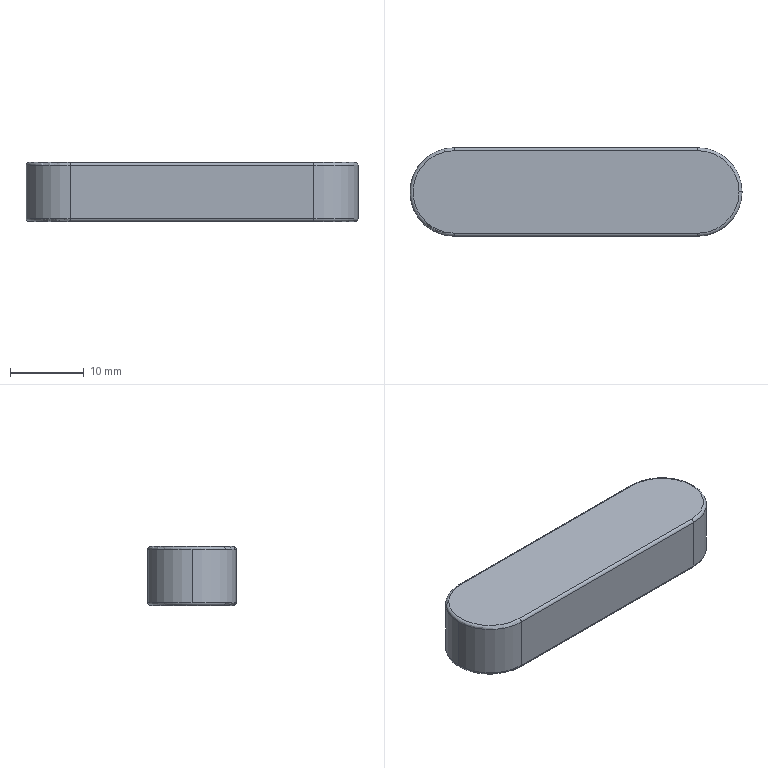Part | SolidWorks | features Extrusion 1, Fillet 1 | 1 solid | 17 faces | box 45 x 12 x 8 mm | volume 4066 mm3 | cylinder 7 | torus 6 | plane 4 | commonest cylinder face diameters 0.8 x4 12 x3
STEP:
#1=CARTESIAN_POINT('',(22.1,0.,0.));
#2=VERTEX_POINT('',#1);
#3=CARTESIAN_POINT('',(16.5,-5.6,0.));
#4=VERTEX_POINT('',#3);
#5=CARTESIAN_POINT('',(16.5,0.,0.));
#6=DIRECTION('',(0.,0.,-1.));
#7=DIRECTION('',(1.,0.,0.));
#8=AXIS2_PLACEMENT_3D('',#5,#6,#7);
#9=CIRCLE('',#8,5.6);
#10=EDGE_CURVE('',#2,#4,#9,.T.);
#11=ORIENTED_EDGE('',*,*,#10,.F.);
#12=CARTESIAN_POINT('',(22.5,0.,0.4));
#13=VERTEX_POINT('',#12);
#14=CARTESIAN_POINT('',(22.1,0.,0.4));
#15=DIRECTION('',(0.,-1.,0.));
#16=DIRECTION('',(0.,0.,-1.));
#17=AXIS2_PLACEMENT_3D('',#14,#15,#16);
#18=CIRCLE('',#17,0.4);
#19=EDGE_CURVE('',#2,#13,#18,.T.);
#20=ORIENTED_EDGE('',*,*,#19,.T.);
#21=CARTESIAN_POINT('',(16.5,-6.,0.4));
#22=VERTEX_POINT('',#21);
#23=CARTESIAN_POINT('',(16.5,0.,0.4));
#24=DIRECTION('',(0.,0.,1.));
#25=DIRECTION('',(1.,0.,0.));
#26=AXIS2_PLACEMENT_3D('',#23,#24,#25);
#27=CIRCLE('',#26,6.);
#28=EDGE_CURVE('',#22,#13,#27,.T.);
#29=ORIENTED_EDGE('',*,*,#28,.F.);
#30=CARTESIAN_POINT('',(16.5,-5.6,0.4));
#31=DIRECTION('',(1.,0.,0.));
#32=DIRECTION('',(0.,0.,-1.));
#33=AXIS2_PLACEMENT_3D('',#30,#31,#32);
#34=CIRCLE('',#33,0.4);
#35=EDGE_CURVE('',#22,#4,#34,.T.);
#36=ORIENTED_EDGE('',*,*,#35,.T.);
#37=EDGE_LOOP('',(#11,#20,#29,#36));
#38=FACE_OUTER_BOUND('',#37,.T.);
#39=CARTESIAN_POINT('',(16.5,0.,0.4));
#40=DIRECTION('',(0.,0.,1.));
#41=DIRECTION('',(1.,0.,0.));
#42=AXIS2_PLACEMENT_3D('',#39,#40,#41);
#43=TOROIDAL_SURFACE('',#42,5.6,0.4);
#44=ADVANCED_FACE('',(#38),#43,.T.);
#45=CARTESIAN_POINT('',(22.5,0.,7.6));
#46=VERTEX_POINT('',#45);
#47=CARTESIAN_POINT('',(16.5,-6.,7.6));
#48=VERTEX_POINT('',#47);
#49=CARTESIAN_POINT('',(16.5,0.,7.6));
#50=DIRECTION('',(0.,0.,-1.));
#51=DIRECTION('',(1.,0.,0.));
#52=AXIS2_PLACEMENT_3D('',#49,#50,#51);
#53=CIRCLE('',#52,6.);
#54=EDGE_CURVE('',#46,#48,#53,.T.);
#55=ORIENTED_EDGE('',*,*,#54,.F.);
#56=CARTESIAN_POINT('',(22.1,0.,8.));
#57=VERTEX_POINT('',#56);
#58=CARTESIAN_POINT('',(22.1,0.,7.6));
#59=DIRECTION('',(0.,-1.,0.));
#60=DIRECTION('',(0.,0.,-1.));
#61=AXIS2_PLACEMENT_3D('',#58,#59,#60);
#62=CIRCLE('',#61,0.4);
#63=EDGE_CURVE('',#46,#57,#62,.T.);
#64=ORIENTED_EDGE('',*,*,#63,.T.);
#65=CARTESIAN_POINT('',(16.5,-5.6,8.));
#66=VERTEX_POINT('',#65);
#67=CARTESIAN_POINT('',(16.5,0.,8.));
#68=DIRECTION('',(0.,0.,1.));
#69=DIRECTION('',(1.,0.,0.));
#70=AXIS2_PLACEMENT_3D('',#67,#68,#69);
#71=CIRCLE('',#70,5.6);
#72=EDGE_CURVE('',#66,#57,#71,.T.);
#73=ORIENTED_EDGE('',*,*,#72,.F.);
#74=CARTESIAN_POINT('',(16.5,-5.6,7.6));
#75=DIRECTION('',(1.,0.,0.));
#76=DIRECTION('',(0.,0.,-1.));
#77=AXIS2_PLACEMENT_3D('',#74,#75,#76);
#78=CIRCLE('',#77,0.4);
#79=EDGE_CURVE('',#66,#48,#78,.T.);
#80=ORIENTED_EDGE('',*,*,#79,.T.);
#81=EDGE_LOOP('',(#55,#64,#73,#80));
#82=FACE_OUTER_BOUND('',#81,.T.);
#83=CARTESIAN_POINT('',(16.5,0.,7.6));
#84=DIRECTION('',(0.,0.,1.));
#85=DIRECTION('',(1.,0.,0.));
#86=AXIS2_PLACEMENT_3D('',#83,#84,#85);
#87=TOROIDAL_SURFACE('',#86,5.6,0.4);
#88=ADVANCED_FACE('',(#82),#87,.T.);
#89=CARTESIAN_POINT('',(-16.5,-6.,7.6));
#90=VERTEX_POINT('',#89);
#91=CARTESIAN_POINT('',(-22.5,0.,7.6));
#92=VERTEX_POINT('',#91);
#93=CARTESIAN_POINT('',(-16.5,0.,7.6));
#94=DIRECTION('',(0.,0.,-1.));
#95=DIRECTION('',(1.,0.,0.));
#96=AXIS2_PLACEMENT_3D('',#93,#94,#95);
#97=CIRCLE('',#96,6.);
#98=EDGE_CURVE('',#90,#92,#97,.T.);
#99=ORIENTED_EDGE('',*,*,#98,.T.);
#100=CARTESIAN_POINT('',(-22.5,0.,0.4));
#101=VERTEX_POINT('',#100);
#102=CARTESIAN_POINT('',(-22.5,0.,8.));
#103=DIRECTION('',(0.,0.,-1.));
#104=VECTOR('',#103,1000.);
#105=LINE('',#102,#104);
#106=EDGE_CURVE('',#92,#101,#105,.T.);
#107=ORIENTED_EDGE('',*,*,#106,.T.);
#108=CARTESIAN_POINT('',(-16.5,-6.,0.4));
#109=VERTEX_POINT('',#108);
#110=CARTESIAN_POINT('',(-16.5,0.,0.4));
#111=DIRECTION('',(0.,0.,1.));
#112=DIRECTION('',(1.,0.,0.));
#113=AXIS2_PLACEMENT_3D('',#110,#111,#112);
#114=CIRCLE('',#113,6.);
#115=EDGE_CURVE('',#101,#109,#114,.T.);
#116=ORIENTED_EDGE('',*,*,#115,.T.);
#117=CARTESIAN_POINT('',(-16.5,-6.,8.));
#118=DIRECTION('',(0.,0.,-1.));
#119=VECTOR('',#118,1000.);
#120=LINE('',#117,#119);
#121=EDGE_CURVE('',#90,#109,#120,.T.);
#122=ORIENTED_EDGE('',*,*,#121,.F.);
#123=EDGE_LOOP('',(#99,#107,#116,#122));
#124=FACE_OUTER_BOUND('',#123,.T.);
#125=CARTESIAN_POINT('',(-16.5,0.,8.));
#126=DIRECTION('',(0.,0.,-1.));
#127=DIRECTION('',(-1.,0.,0.));
#128=AXIS2_PLACEMENT_3D('',#125,#126,#127);
#129=CYLINDRICAL_SURFACE('',#128,6.);
#130=ADVANCED_FACE('',(#124),#129,.T.);
#131=ORIENTED_EDGE('',*,*,#106,.F.);
#132=CARTESIAN_POINT('',(-16.5,6.,7.6));
#133=VERTEX_POINT('',#132);
#134=CARTESIAN_POINT('',(-16.5,0.,7.6));
#135=DIRECTION('',(0.,0.,-1.));
#136=DIRECTION('',(1.,0.,0.));
#137=AXIS2_PLACEMENT_3D('',#134,#135,#136);
#138=CIRCLE('',#137,6.);
#139=EDGE_CURVE('',#92,#133,#138,.T.);
#140=ORIENTED_EDGE('',*,*,#139,.T.);
#141=CARTESIAN_POINT('',(-16.5,6.,0.4));
#142=VERTEX_POINT('',#141);
#143=CARTESIAN_POINT('',(-16.5,6.,8.));
#144=DIRECTION('',(0.,0.,-1.));
#145=VECTOR('',#144,1000.);
#146=LINE('',#143,#145);
#147=EDGE_CURVE('',#133,#142,#146,.T.);
#148=ORIENTED_EDGE('',*,*,#147,.T.);
#149=CARTESIAN_POINT('',(-16.5,0.,0.4));
#150=DIRECTION('',(0.,0.,1.));
#151=DIRECTION('',(1.,0.,0.));
#152=AXIS2_PLACEMENT_3D('',#149,#150,#151);
#153=CIRCLE('',#152,6.);
#154=EDGE_CURVE('',#142,#101,#153,.T.);
#155=ORIENTED_EDGE('',*,*,#154,.T.);
#156=EDGE_LOOP('',(#131,#140,#148,#155));
#157=FACE_OUTER_BOUND('',#156,.T.);
#158=CARTESIAN_POINT('',(-16.5,0.,8.));
#159=DIRECTION('',(0.,0.,-1.));
#160=DIRECTION('',(-1.,0.,0.));
#161=AXIS2_PLACEMENT_3D('',#158,#159,#160);
#162=CYLINDRICAL_SURFACE('',#161,6.);
#163=ADVANCED_FACE('',(#157),#162,.T.);
#164=CARTESIAN_POINT('',(16.5,-6.,8.));
#165=DIRECTION('',(0.,0.,-1.));
#166=VECTOR('',#165,1000.);
#167=LINE('',#164,#166);
#168=EDGE_CURVE('',#48,#22,#167,.T.);
#169=ORIENTED_EDGE('',*,*,#168,.F.);
#170=CARTESIAN_POINT('',(-16.5,-6.,7.6));
#171=DIRECTION('',(-1.,0.,0.));
#172=VECTOR('',#171,1000.);
#173=LINE('',#170,#172);
#174=EDGE_CURVE('',#48,#90,#173,.T.);
#175=ORIENTED_EDGE('',*,*,#174,.T.);
#176=ORIENTED_EDGE('',*,*,#121,.T.);
#177=CARTESIAN_POINT('',(-16.5,-6.,0.4));
#178=DIRECTION('',(1.,0.,0.));
#179=VECTOR('',#178,1000.);
#180=LINE('',#177,#179);
#181=EDGE_CURVE('',#109,#22,#180,.T.);
#182=ORIENTED_EDGE('',*,*,#181,.T.);
#183=EDGE_LOOP('',(#169,#175,#176,#182));
#184=FACE_OUTER_BOUND('',#183,.T.);
#185=CARTESIAN_POINT('',(-16.5,-6.,8.));
#186=DIRECTION('',(0.,1.,0.));
#187=DIRECTION('',(-1.,0.,0.));
#188=AXIS2_PLACEMENT_3D('',#185,#186,#187);
#189=PLANE('',#188);
#190=ADVANCED_FACE('',(#184),#189,.F.);
#191=CARTESIAN_POINT('',(16.5,6.,7.6));
#192=VERTEX_POINT('',#191);
#193=CARTESIAN_POINT('',(16.5,6.,0.4));
#194=VERTEX_POINT('',#193);
#195=CARTESIAN_POINT('',(16.5,6.,8.));
#196=DIRECTION('',(0.,0.,-1.));
#197=VECTOR('',#196,1000.);
#198=LINE('',#195,#197);
#199=EDGE_CURVE('',#192,#194,#198,.T.);
#200=ORIENTED_EDGE('',*,*,#199,.F.);
#201=CARTESIAN_POINT('',(16.5,0.,7.6));
#202=DIRECTION('',(0.,0.,-1.));
#203=DIRECTION('',(1.,0.,0.));
#204=AXIS2_PLACEMENT_3D('',#201,#202,#203);
#205=CIRCLE('',#204,6.);
#206=EDGE_CURVE('',#192,#46,#205,.T.);
#207=ORIENTED_EDGE('',*,*,#206,.T.);
#208=ORIENTED_EDGE('',*,*,#54,.T.);
#209=ORIENTED_EDGE('',*,*,#168,.T.);
#210=ORIENTED_EDGE('',*,*,#28,.T.);
#211=CARTESIAN_POINT('',(16.5,0.,0.4));
#212=DIRECTION('',(0.,0.,1.));
#213=DIRECTION('',(1.,0.,0.));
#214=AXIS2_PLACEMENT_3D('',#211,#212,#213);
#215=CIRCLE('',#214,6.);
#216=EDGE_CURVE('',#13,#194,#215,.T.);
#217=ORIENTED_EDGE('',*,*,#216,.T.);
#218=EDGE_LOOP('',(#200,#207,#208,#209,#210,#217));
#219=FACE_OUTER_BOUND('',#218,.T.);
#220=CARTESIAN_POINT('',(16.5,0.,8.));
#221=DIRECTION('',(0.,0.,-1.));
#222=DIRECTION('',(-1.,0.,0.));
#223=AXIS2_PLACEMENT_3D('',#220,#221,#222);
#224=CYLINDRICAL_SURFACE('',#223,6.);
#225=ADVANCED_FACE('',(#219),#224,.T.);
#226=ORIENTED_EDGE('',*,*,#147,.F.);
#227=CARTESIAN_POINT('',(16.5,6.,7.6));
#228=DIRECTION('',(1.,0.,0.));
#229=VECTOR('',#228,1000.);
#230=LINE('',#227,#229);
#231=EDGE_CURVE('',#133,#192,#230,.T.);
#232=ORIENTED_EDGE('',*,*,#231,.T.);
#233=ORIENTED_EDGE('',*,*,#199,.T.);
#234=CARTESIAN_POINT('',(-16.5,6.,0.4));
#235=DIRECTION('',(-1.,0.,0.));
#236=VECTOR('',#235,1000.);
#237=LINE('',#234,#236);
#238=EDGE_CURVE('',#194,#142,#237,.T.);
#239=ORIENTED_EDGE('',*,*,#238,.T.);
#240=EDGE_LOOP('',(#226,#232,#233,#239));
#241=FACE_OUTER_BOUND('',#240,.T.);
#242=CARTESIAN_POINT('',(-16.5,6.,8.));
#243=DIRECTION('',(0.,-1.,0.));
#244=DIRECTION('',(1.,0.,0.));
#245=AXIS2_PLACEMENT_3D('',#242,#243,#244);
#246=PLANE('',#245);
#247=ADVANCED_FACE('',(#241),#246,.F.);
#248=CARTESIAN_POINT('',(-16.5,-5.6,8.));
#249=VERTEX_POINT('',#248);
#250=CARTESIAN_POINT('',(16.5,-5.6,8.));
#251=DIRECTION('',(1.,0.,0.));
#252=VECTOR('',#251,1000.);
#253=LINE('',#250,#252);
#254=EDGE_CURVE('',#249,#66,#253,.T.);
#255=ORIENTED_EDGE('',*,*,#254,.T.);
#256=ORIENTED_EDGE('',*,*,#72,.T.);
#257=CARTESIAN_POINT('',(16.5,5.6,8.));
#258=VERTEX_POINT('',#257);
#259=CARTESIAN_POINT('',(16.5,0.,8.));
#260=DIRECTION('',(0.,0.,1.));
#261=DIRECTION('',(1.,0.,0.));
#262=AXIS2_PLACEMENT_3D('',#259,#260,#261);
#263=CIRCLE('',#262,5.6);
#264=EDGE_CURVE('',#57,#258,#263,.T.);
#265=ORIENTED_EDGE('',*,*,#264,.T.);
#266=CARTESIAN_POINT('',(-16.5,5.6,8.));
#267=VERTEX_POINT('',#266);
#268=CARTESIAN_POINT('',(-16.5,5.6,8.));
#269=DIRECTION('',(-1.,0.,0.));
#270=VECTOR('',#269,1000.);
#271=LINE('',#268,#270);
#272=EDGE_CURVE('',#258,#267,#271,.T.);
#273=ORIENTED_EDGE('',*,*,#272,.T.);
#274=CARTESIAN_POINT('',(-16.5,0.,8.));
#275=DIRECTION('',(0.,0.,1.));
#276=DIRECTION('',(1.,0.,0.));
#277=AXIS2_PLACEMENT_3D('',#274,#275,#276);
#278=CIRCLE('',#277,5.6);
#279=EDGE_CURVE('',#267,#249,#278,.T.);
#280=ORIENTED_EDGE('',*,*,#279,.T.);
#281=EDGE_LOOP('',(#255,#256,#265,#273,#280));
#282=FACE_OUTER_BOUND('',#281,.T.);
#283=CARTESIAN_POINT('',(-16.5,0.,8.));
#284=DIRECTION('',(0.,0.,1.));
#285=DIRECTION('',(1.,0.,0.));
#286=AXIS2_PLACEMENT_3D('',#283,#284,#285);
#287=PLANE('',#286);
#288=ADVANCED_FACE('',(#282),#287,.T.);
#289=CARTESIAN_POINT('',(-16.5,5.6,0.));
#290=VERTEX_POINT('',#289);
#291=CARTESIAN_POINT('',(16.5,5.6,0.));
#292=VERTEX_POINT('',#291);
#293=CARTESIAN_POINT('',(-16.5,5.6,0.));
#294=DIRECTION('',(1.,0.,0.));
#295=VECTOR('',#294,1000.);
#296=LINE('',#293,#295);
#297=EDGE_CURVE('',#290,#292,#296,.T.);
#298=ORIENTED_EDGE('',*,*,#297,.T.);
#299=CARTESIAN_POINT('',(16.5,0.,0.));
#300=DIRECTION('',(0.,0.,-1.));
#301=DIRECTION('',(1.,0.,0.));
#302=AXIS2_PLACEMENT_3D('',#299,#300,#301);
#303=CIRCLE('',#302,5.6);
#304=EDGE_CURVE('',#292,#2,#303,.T.);
#305=ORIENTED_EDGE('',*,*,#304,.T.);
#306=ORIENTED_EDGE('',*,*,#10,.T.);
#307=CARTESIAN_POINT('',(-16.5,-5.6,0.));
#308=VERTEX_POINT('',#307);
#309=CARTESIAN_POINT('',(-16.5,-5.6,0.));
#310=DIRECTION('',(-1.,0.,0.));
#311=VECTOR('',#310,1000.);
#312=LINE('',#309,#311);
#313=EDGE_CURVE('',#4,#308,#312,.T.);
#314=ORIENTED_EDGE('',*,*,#313,.T.);
#315=CARTESIAN_POINT('',(-16.5,0.,0.));
#316=DIRECTION('',(0.,0.,-1.));
#317=DIRECTION('',(1.,0.,0.));
#318=AXIS2_PLACEMENT_3D('',#315,#316,#317);
#319=CIRCLE('',#318,5.6);
#320=EDGE_CURVE('',#308,#290,#319,.T.);
#321=ORIENTED_EDGE('',*,*,#320,.T.);
#322=EDGE_LOOP('',(#298,#305,#306,#314,#321));
#323=FACE_OUTER_BOUND('',#322,.T.);
#324=CARTESIAN_POINT('',(-16.5,0.,0.));
#325=DIRECTION('',(0.,0.,1.));
#326=DIRECTION('',(1.,0.,0.));
#327=AXIS2_PLACEMENT_3D('',#324,#325,#326);
#328=PLANE('',#327);
#329=ADVANCED_FACE('',(#323),#328,.F.);
#330=CARTESIAN_POINT('',(-16.5,5.6,7.6));
#331=DIRECTION('',(1.,0.,0.));
#332=DIRECTION('',(0.,0.,-1.));
#333=AXIS2_PLACEMENT_3D('',#330,#331,#332);
#334=CIRCLE('',#333,0.4);
#335=EDGE_CURVE('',#133,#267,#334,.T.);
#336=ORIENTED_EDGE('',*,*,#335,.F.);
#337=ORIENTED_EDGE('',*,*,#139,.F.);
#338=ORIENTED_EDGE('',*,*,#98,.F.);
#339=CARTESIAN_POINT('',(-16.5,-5.6,7.6));
#340=DIRECTION('',(1.,0.,0.));
#341=DIRECTION('',(0.,0.,-1.));
#342=AXIS2_PLACEMENT_3D('',#339,#340,#341);
#343=CIRCLE('',#342,0.4);
#344=EDGE_CURVE('',#249,#90,#343,.T.);
#345=ORIENTED_EDGE('',*,*,#344,.F.);
#346=ORIENTED_EDGE('',*,*,#279,.F.);
#347=EDGE_LOOP('',(#336,#337,#338,#345,#346));
#348=FACE_OUTER_BOUND('',#347,.T.);
#349=CARTESIAN_POINT('',(-16.5,0.,7.6));
#350=DIRECTION('',(0.,0.,1.));
#351=DIRECTION('',(1.,0.,0.));
#352=AXIS2_PLACEMENT_3D('',#349,#350,#351);
#353=TOROIDAL_SURFACE('',#352,5.6,0.4);
#354=ADVANCED_FACE('',(#348),#353,.T.);
#355=ORIENTED_EDGE('',*,*,#344,.T.);
#356=ORIENTED_EDGE('',*,*,#174,.F.);
#357=ORIENTED_EDGE('',*,*,#79,.F.);
#358=ORIENTED_EDGE('',*,*,#254,.F.);
#359=EDGE_LOOP('',(#355,#356,#357,#358));
#360=FACE_OUTER_BOUND('',#359,.T.);
#361=CARTESIAN_POINT('',(-16.5,-5.6,7.6));
#362=DIRECTION('',(-1.,0.,0.));
#363=DIRECTION('',(0.,-1.,0.));
#364=AXIS2_PLACEMENT_3D('',#361,#362,#363);
#365=CYLINDRICAL_SURFACE('',#364,0.4);
#366=ADVANCED_FACE('',(#360),#365,.T.);
#367=ORIENTED_EDGE('',*,*,#335,.T.);
#368=ORIENTED_EDGE('',*,*,#272,.F.);
#369=CARTESIAN_POINT('',(16.5,5.6,7.6));
#370=DIRECTION('',(1.,0.,0.));
#371=DIRECTION('',(0.,0.,-1.));
#372=AXIS2_PLACEMENT_3D('',#369,#370,#371);
#373=CIRCLE('',#372,0.4);
#374=EDGE_CURVE('',#192,#258,#373,.T.);
#375=ORIENTED_EDGE('',*,*,#374,.F.);
#376=ORIENTED_EDGE('',*,*,#231,.F.);
#377=EDGE_LOOP('',(#367,#368,#375,#376));
#378=FACE_OUTER_BOUND('',#377,.T.);
#379=CARTESIAN_POINT('',(-16.5,5.6,7.6));
#380=DIRECTION('',(1.,0.,0.));
#381=DIRECTION('',(0.,1.,0.));
#382=AXIS2_PLACEMENT_3D('',#379,#380,#381);
#383=CYLINDRICAL_SURFACE('',#382,0.4);
#384=ADVANCED_FACE('',(#378),#383,.T.);
#385=ORIENTED_EDGE('',*,*,#63,.F.);
#386=ORIENTED_EDGE('',*,*,#206,.F.);
#387=ORIENTED_EDGE('',*,*,#374,.T.);
#388=ORIENTED_EDGE('',*,*,#264,.F.);
#389=EDGE_LOOP('',(#385,#386,#387,#388));
#390=FACE_OUTER_BOUND('',#389,.T.);
#391=CARTESIAN_POINT('',(16.5,0.,7.6));
#392=DIRECTION('',(0.,0.,1.));
#393=DIRECTION('',(1.,0.,0.));
#394=AXIS2_PLACEMENT_3D('',#391,#392,#393);
#395=TOROIDAL_SURFACE('',#394,5.6,0.4);
#396=ADVANCED_FACE('',(#390),#395,.T.);
#397=CARTESIAN_POINT('',(-16.5,5.6,0.4));
#398=DIRECTION('',(1.,0.,0.));
#399=DIRECTION('',(0.,0.,-1.));
#400=AXIS2_PLACEMENT_3D('',#397,#398,#399);
#401=CIRCLE('',#400,0.4);
#402=EDGE_CURVE('',#290,#142,#401,.T.);
#403=ORIENTED_EDGE('',*,*,#402,.F.);
#404=ORIENTED_EDGE('',*,*,#320,.F.);
#405=CARTESIAN_POINT('',(-16.5,-5.6,0.4));
#406=DIRECTION('',(1.,0.,0.));
#407=DIRECTION('',(0.,0.,-1.));
#408=AXIS2_PLACEMENT_3D('',#405,#406,#407);
#409=CIRCLE('',#408,0.4);
#410=EDGE_CURVE('',#109,#308,#409,.T.);
#411=ORIENTED_EDGE('',*,*,#410,.F.);
#412=ORIENTED_EDGE('',*,*,#115,.F.);
#413=ORIENTED_EDGE('',*,*,#154,.F.);
#414=EDGE_LOOP('',(#403,#404,#411,#412,#413));
#415=FACE_OUTER_BOUND('',#414,.T.);
#416=CARTESIAN_POINT('',(-16.5,0.,0.4));
#417=DIRECTION('',(0.,0.,1.));
#418=DIRECTION('',(1.,0.,0.));
#419=AXIS2_PLACEMENT_3D('',#416,#417,#418);
#420=TOROIDAL_SURFACE('',#419,5.6,0.4);
#421=ADVANCED_FACE('',(#415),#420,.T.);
#422=ORIENTED_EDGE('',*,*,#410,.T.);
#423=ORIENTED_EDGE('',*,*,#313,.F.);
#424=ORIENTED_EDGE('',*,*,#35,.F.);
#425=ORIENTED_EDGE('',*,*,#181,.F.);
#426=EDGE_LOOP('',(#422,#423,#424,#425));
#427=FACE_OUTER_BOUND('',#426,.T.);
#428=CARTESIAN_POINT('',(-16.5,-5.6,0.4));
#429=DIRECTION('',(1.,0.,0.));
#430=DIRECTION('',(0.,1.,0.));
#431=AXIS2_PLACEMENT_3D('',#428,#429,#430);
#432=CYLINDRICAL_SURFACE('',#431,0.4);
#433=ADVANCED_FACE('',(#427),#432,.T.);
#434=ORIENTED_EDGE('',*,*,#402,.T.);
#435=ORIENTED_EDGE('',*,*,#238,.F.);
#436=CARTESIAN_POINT('',(16.5,5.6,0.4));
#437=DIRECTION('',(1.,0.,0.));
#438=DIRECTION('',(0.,0.,-1.));
#439=AXIS2_PLACEMENT_3D('',#436,#437,#438);
#440=CIRCLE('',#439,0.4);
#441=EDGE_CURVE('',#292,#194,#440,.T.);
#442=ORIENTED_EDGE('',*,*,#441,.F.);
#443=ORIENTED_EDGE('',*,*,#297,.F.);
#444=EDGE_LOOP('',(#434,#435,#442,#443));
#445=FACE_OUTER_BOUND('',#444,.T.);
#446=CARTESIAN_POINT('',(-16.5,5.6,0.4));
#447=DIRECTION('',(-1.,0.,0.));
#448=DIRECTION('',(0.,-1.,0.));
#449=AXIS2_PLACEMENT_3D('',#446,#447,#448);
#450=CYLINDRICAL_SURFACE('',#449,0.4);
#451=ADVANCED_FACE('',(#445),#450,.T.);
#452=ORIENTED_EDGE('',*,*,#19,.F.);
#453=ORIENTED_EDGE('',*,*,#304,.F.);
#454=ORIENTED_EDGE('',*,*,#441,.T.);
#455=ORIENTED_EDGE('',*,*,#216,.F.);
#456=EDGE_LOOP('',(#452,#453,#454,#455));
#457=FACE_OUTER_BOUND('',#456,.T.);
#458=CARTESIAN_POINT('',(16.5,0.,0.4));
#459=DIRECTION('',(0.,0.,1.));
#460=DIRECTION('',(1.,0.,0.));
#461=AXIS2_PLACEMENT_3D('',#458,#459,#460);
#462=TOROIDAL_SURFACE('',#461,5.6,0.4);
#463=ADVANCED_FACE('',(#457),#462,.T.);
#464=CLOSED_SHELL('',(#44,#88,#130,#163,#190,#225,#247,#288,#329,#354,#366,#384,#396,#421,#433,#451,#463));
#465=MANIFOLD_SOLID_BREP('',#464);
#466=CARTESIAN_POINT('',(0.,0.,0.));
#467=DIRECTION('',(0.,0.,1.));
#468=DIRECTION('',(1.,0.,0.));
#469=AXIS2_PLACEMENT_3D('',#466,#467,#468);
#470=(LENGTH_UNIT()NAMED_UNIT(*)SI_UNIT(.MILLI.,.METRE.));
#471=UNCERTAINTY_MEASURE_WITH_UNIT(LENGTH_MEASURE(0.00001),#470,'','');
#472=(NAMED_UNIT(*)PLANE_ANGLE_UNIT()SI_UNIT($,.RADIAN.));
#473=(NAMED_UNIT(*)SI_UNIT($,.STERADIAN.)SOLID_ANGLE_UNIT());
#474=(GEOMETRIC_REPRESENTATION_CONTEXT(3)GLOBAL_UNCERTAINTY_ASSIGNED_CONTEXT((#471))GLOBAL_UNIT_ASSIGNED_CONTEXT((#470,#472,#473))REPRESENTATION_CONTEXT('',''));
#475=ADVANCED_BREP_SHAPE_REPRESENTATION('',(#465,#469),#474);